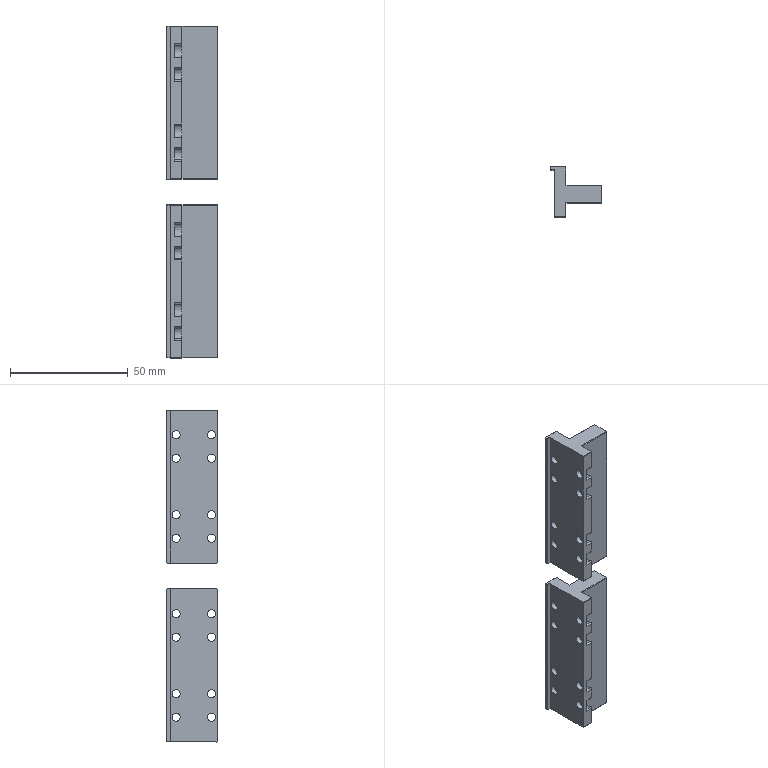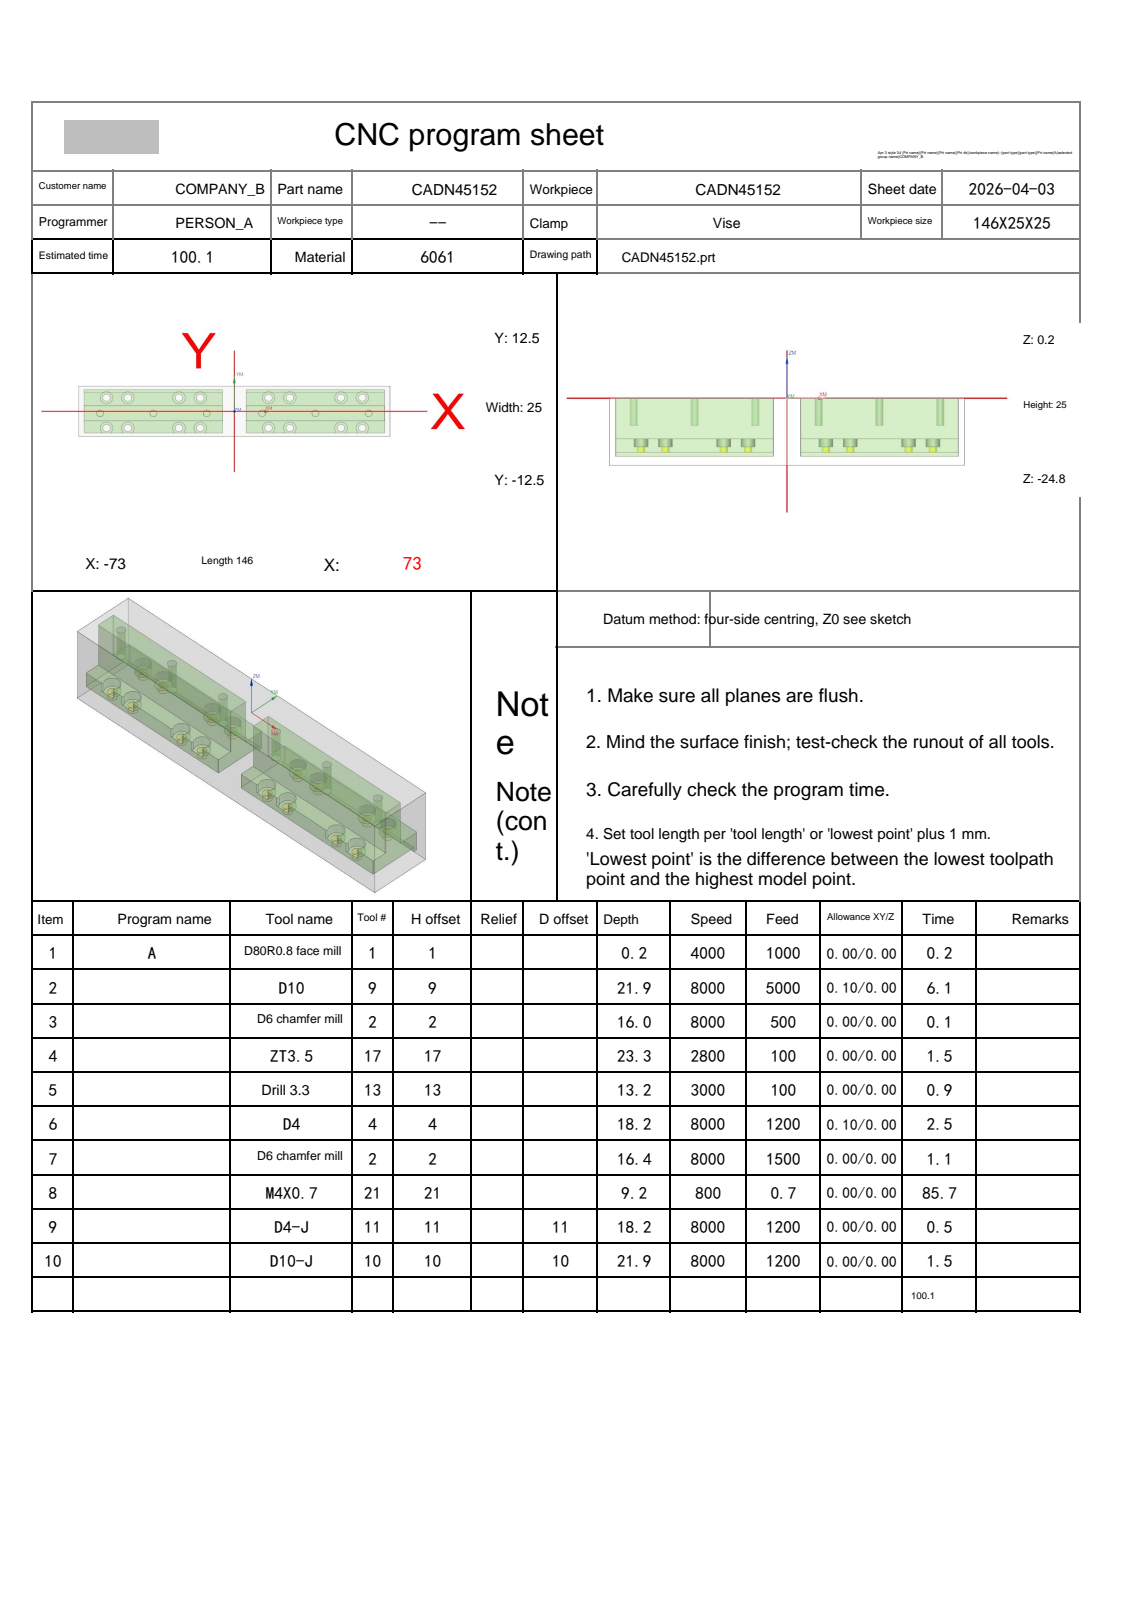NC program | NX | posted by the shop | part box 21.5 x 21.5 x 141 mm
Lines 36 to 798 of 7245:
N2 T09 M06
(D10  D=10. R=0. H=09 ce=0.10 di=0.00)
G00 G90 G54 X-38. Y-15.85 M03 S8000
G43 H09 Z20.
M08
Z.5
G01 X-70.3 Z.375 F5000.
G02 X-73.906 Y-14.356 Z.359 I0.0 J5.1
G01 X-74.106 Y-14.156 Z.358
G02 X-75.6 Y-10.55 Z.343 I3.606 J3.606
G01 Y10.55 Z.261
G02 X-74.106 Y14.156 Z.245 I5.1 J0.0
G01 X-73.906 Y14.356 Z.244
G02 X-70.3 Y15.85 Z.229 I3.606 J-3.606
G01 X-5.7 Z-.022
G02 X-2.094 Y14.356 Z-.037 I0.0 J-5.1
G01 X-1.894 Y14.156 Z-.038
G02 X-.4 Y10.55 Z-.054 I-3.606 J-3.606
G01 Y-10.55 Z-.136
G02 X-1.894 Y-14.156 Z-.151 I-5.1 J0.0
G01 X-2.094 Y-14.356 Z-.152
G02 X-5.7 Y-15.85 Z-.168 I-3.606 J3.606
G01 X-70.3 Z-.418
G02 X-73.906 Y-14.356 Z-.434 I0.0 J5.1
G01 X-74.106 Y-14.156 Z-.435
G02 X-75.6 Y-10.55 Z-.45 I3.606 J3.606
G01 Y10.55 Z-.532
G02 X-74.106 Y14.156 Z-.547 I5.1 J0.0
G01 X-73.906 Y14.356 Z-.549
G02 X-70.3 Y15.85 Z-.564 I3.606 J-3.606
G01 X-5.7 Z-.814
G02 X-2.094 Y14.356 Z-.83 I0.0 J-5.1
G01 X-1.894 Y14.156 Z-.831
G02 X-.4 Y10.55 Z-.847 I-3.606 J-3.606
G01 Y-10.55 Z-.928
G02 X-1.894 Y-14.156 Z-.944 I-5.1 J0.0
G01 X-2.094 Y-14.356 Z-.945
G02 X-5.7 Y-15.85 Z-.961 I-3.606 J3.606
G01 X-70.3 Z-1.211
G02 X-73.906 Y-14.356 Z-1.226 I0.0 J5.1
G01 X-74.106 Y-14.156 Z-1.228
G02 X-75.6 Y-10.55 Z-1.243 I3.606 J3.606
G01 Y10.55 Z-1.325
G02 X-74.106 Y14.156 Z-1.34 I5.1 J0.0
G01 X-73.906 Y14.356 Z-1.341
G02 X-70.3 Y15.85 Z-1.357 I3.606 J-3.606
G01 X-5.7 Z-1.607
G02 X-2.094 Y14.356 Z-1.623 I0.0 J-5.1
G01 X-1.894 Y14.156 Z-1.624
G02 X-.4 Y10.55 Z-1.639 I-3.606 J-3.606
G01 Y-10.55 Z-1.721
G02 X-1.894 Y-14.156 Z-1.737 I-5.1 J0.0
G01 X-2.094 Y-14.356 Z-1.738
G02 X-5.7 Y-15.85 Z-1.753 I-3.606 J3.606
G01 X-70.3 Z-2.004
G02 X-73.906 Y-14.356 Z-2.019 I0.0 J5.1
G01 X-74.106 Y-14.156 Z-2.02
G02 X-75.6 Y-10.55 Z-2.036 I3.606 J3.606
G01 Y10.55 Z-2.118
G02 X-74.106 Y14.156 Z-2.133 I5.1 J0.0
G01 X-73.906 Y14.356 Z-2.134
G02 X-70.3 Y15.85 Z-2.15 I3.606 J-3.606
G01 X-5.7 Z-2.4
G02 X-2.094 Y14.356 Z-2.416 I0.0 J-5.1
G01 X-1.894 Y14.156 Z-2.417
G02 X-.4 Y10.55 Z-2.432 I-3.606 J-3.606
G01 Y-10.55 Z-2.514
G02 X-1.894 Y-14.156 Z-2.53 I-5.1 J0.0
G01 X-2.094 Y-14.356 Z-2.531
G02 X-5.7 Y-15.85 Z-2.546 I-3.606 J3.606
G01 X-70.3 Z-2.797
G02 X-73.906 Y-14.356 Z-2.812 I0.0 J5.1
G01 X-74.106 Y-14.156 Z-2.813
G02 X-75.6 Y-10.55 Z-2.829 I3.606 J3.606
G01 Y10.55 Z-2.911
G02 X-74.106 Y14.156 Z-2.926 I5.1 J0.0
G01 X-73.906 Y14.356 Z-2.927
G02 X-70.3 Y15.85 Z-2.943 I3.606 J-3.606
G01 X-5.7 Z-3.193
G02 X-2.094 Y14.356 Z-3.209 I0.0 J-5.1
G01 X-1.894 Y14.156 Z-3.21
G02 X-.4 Y10.55 Z-3.225 I-3.606 J-3.606
G01 Y-10.55 Z-3.307
G02 X-1.894 Y-14.156 Z-3.322 I-5.1 J0.0
G01 X-2.094 Y-14.356 Z-3.324
G02 X-5.7 Y-15.85 Z-3.339 I-3.606 J3.606
G01 X-70.3 Z-3.589
G02 X-73.906 Y-14.356 Z-3.605 I0.0 J5.1
G01 X-74.106 Y-14.156 Z-3.606
G02 X-75.6 Y-10.55 Z-3.622 I3.606 J3.606
G01 Y10.55 Z-3.703
G02 X-74.106 Y14.156 Z-3.719 I5.1 J0.0
G01 X-73.906 Y14.356 Z-3.72
G02 X-70.3 Y15.85 Z-3.736 I3.606 J-3.606
G01 X-5.7 Z-3.986
G02 X-2.094 Y14.356 Z-4.001 I0.0 J-5.1
G01 X-1.894 Y14.156 Z-4.003
G02 X-.4 Y10.55 Z-4.018 I-3.606 J-3.606
G01 Y-10.55 Z-4.1
G02 X-1.894 Y-14.156 Z-4.115 I-5.1 J0.0
G01 X-2.094 Y-14.356 Z-4.116
G02 X-5.7 Y-15.85 Z-4.132 I-3.606 J3.606
G01 X-70.3 Z-4.382
G02 X-73.906 Y-14.356 Z-4.398 I0.0 J5.1
G01 X-74.106 Y-14.156 Z-4.399
G02 X-75.6 Y-10.55 Z-4.414 I3.606 J3.606
G01 Y10.55 Z-4.496
G02 X-74.106 Y14.156 Z-4.512 I5.1 J0.0
G01 X-73.906 Y14.356 Z-4.513
G02 X-70.3 Y15.85 Z-4.528 I3.606 J-3.606
G01 X-5.7 Z-4.779
G02 X-2.094 Y14.356 Z-4.794 I0.0 J-5.1
G01 X-1.894 Y14.156 Z-4.795
G02 X-.4 Y10.55 Z-4.811 I-3.606 J-3.606
G01 Y-10.55 Z-4.893
G02 X-1.894 Y-14.156 Z-4.908 I-5.1 J0.0
G01 X-2.094 Y-14.356 Z-4.909
G02 X-5.7 Y-15.85 Z-4.925 I-3.606 J3.606
G01 X-70.3 Z-5.175
G02 X-73.906 Y-14.356 Z-5.191 I0.0 J5.1
G01 X-74.106 Y-14.156 Z-5.192
G02 X-75.6 Y-10.55 Z-5.207 I3.606 J3.606
G01 Y10.55 Z-5.289
G02 X-74.106 Y14.156 Z-5.305 I5.1 J0.0
G01 X-73.906 Y14.356 Z-5.306
G02 X-70.3 Y15.85 Z-5.321 I3.606 J-3.606
G01 X-5.7 Z-5.572
G02 X-2.094 Y14.356 Z-5.587 I0.0 J-5.1
G01 X-1.894 Y14.156 Z-5.588
G02 X-.4 Y10.55 Z-5.604 I-3.606 J-3.606
G01 Y-10.55 Z-5.686
G02 X-1.894 Y-14.156 Z-5.701 I-5.1 J0.0
G01 X-2.094 Y-14.356 Z-5.702
G02 X-5.7 Y-15.85 Z-5.718 I-3.606 J3.606
G01 X-70.3 Z-5.968
G02 X-73.906 Y-14.356 Z-5.984 I0.0 J5.1
G01 X-74.106 Y-14.156 Z-5.985
G02 X-75.6 Y-10.55 Z-6. I3.606 J3.606
G01 Y10.55 Z-6.082
G02 X-74.106 Y14.156 Z-6.097 I5.1 J0.0
G01 X-73.906 Y14.356 Z-6.099
G02 X-70.3 Y15.85 Z-6.114 I3.606 J-3.606
G01 X-5.7 Z-6.364
G02 X-2.094 Y14.356 Z-6.38 I0.0 J-5.1
G01 X-1.894 Y14.156 Z-6.381
G02 X-.4 Y10.55 Z-6.397 I-3.606 J-3.606
G01 Y-10.55 Z-6.478
G02 X-1.894 Y-14.156 Z-6.494 I-5.1 J0.0
G01 X-2.094 Y-14.356 Z-6.495
G02 X-5.7 Y-15.85 Z-6.511 I-3.606 J3.606
G01 X-70.3 Z-6.761
G02 X-73.906 Y-14.356 Z-6.776 I0.0 J5.1
G01 X-74.106 Y-14.156 Z-6.778
G02 X-75.6 Y-10.55 Z-6.793 I3.606 J3.606
G01 Y10.55 Z-6.875
G02 X-74.106 Y14.156 Z-6.89 I5.1 J0.0
G01 X-73.906 Y14.356 Z-6.891
G02 X-70.3 Y15.85 Z-6.907 I3.606 J-3.606
G01 X-5.7 Z-7.157
G02 X-2.094 Y14.356 Z-7.173 I0.0 J-5.1
G01 X-1.894 Y14.156 Z-7.174
G02 X-.4 Y10.55 Z-7.189 I-3.606 J-3.606
G01 Y-10.55 Z-7.271
G02 X-1.894 Y-14.156 Z-7.287 I-5.1 J0.0
G01 X-2.094 Y-14.356 Z-7.288
G02 X-5.7 Y-15.85 Z-7.303 I-3.606 J3.606
G01 X-70.3 Z-7.554
G02 X-73.906 Y-14.356 Z-7.569 I0.0 J5.1
G01 X-74.106 Y-14.156 Z-7.57
G02 X-75.6 Y-10.55 Z-7.586 I3.606 J3.606
G01 Y10.55 Z-7.668
G02 X-74.106 Y14.156 Z-7.683 I5.1 J0.0
G01 X-73.906 Y14.356 Z-7.684
G02 X-70.3 Y15.85 Z-7.7 I3.606 J-3.606
G01 X-5.7 Z-7.95
G02 X-2.094 Y14.356 Z-7.966 I0.0 J-5.1
G01 X-1.894 Y14.156 Z-7.967
G02 X-.4 Y10.55 Z-7.982 I-3.606 J-3.606
G01 Y-10.55 Z-8.064
G02 X-1.894 Y-14.156 Z-8.08 I-5.1 J0.0
G01 X-2.094 Y-14.356 Z-8.081
G02 X-5.7 Y-15.85 Z-8.096 I-3.606 J3.606
G01 X-70.3 Z-8.347
G02 X-73.906 Y-14.356 Z-8.362 I0.0 J5.1
G01 X-74.106 Y-14.156 Z-8.363
G02 X-75.6 Y-10.55 Z-8.379 I3.606 J3.606
G01 Y10.55 Z-8.461
G02 X-74.106 Y14.156 Z-8.476 I5.1 J0.0
G01 X-73.906 Y14.356 Z-8.477
G02 X-70.3 Y15.85 Z-8.493 I3.606 J-3.606
G01 X-5.7 Z-8.743
G02 X-2.094 Y14.356 Z-8.759 I0.0 J-5.1
G01 X-1.894 Y14.156 Z-8.76
G02 X-.4 Y10.55 Z-8.775 I-3.606 J-3.606
G01 Y-10.55 Z-8.857
G02 X-1.894 Y-14.156 Z-8.872 I-5.1 J0.0
G01 X-2.094 Y-14.356 Z-8.874
G02 X-5.7 Y-15.85 Z-8.889 I-3.606 J3.606
G01 X-70.3 Z-9.139
G02 X-73.906 Y-14.356 Z-9.155 I0.0 J5.1
G01 X-74.106 Y-14.156 Z-9.156
G02 X-75.6 Y-10.55 Z-9.172 I3.606 J3.606
G01 Y10.55 Z-9.253
G02 X-74.106 Y14.156 Z-9.269 I5.1 J0.0
G01 X-73.906 Y14.356 Z-9.27
G02 X-70.3 Y15.85 Z-9.286 I3.606 J-3.606
G01 X-5.7 Z-9.536
G02 X-2.094 Y14.356 Z-9.551 I0.0 J-5.1
G01 X-1.894 Y14.156 Z-9.553
G02 X-.4 Y10.55 Z-9.568 I-3.606 J-3.606
G01 Y-10.55 Z-9.65
G02 X-1.894 Y-14.156 Z-9.665 I-5.1 J0.0
G01 X-2.094 Y-14.356 Z-9.666
G02 X-5.7 Y-15.85 Z-9.682 I-3.606 J3.606
G01 X-70.3 Z-9.932
G02 X-73.906 Y-14.356 Z-9.948 I0.0 J5.1
G01 X-74.106 Y-14.156 Z-9.949
G02 X-75.6 Y-10.55 Z-9.964 I3.606 J3.606
G01 Y10.55 Z-10.046
G02 X-74.106 Y14.156 Z-10.062 I5.1 J0.0
G01 X-73.906 Y14.356 Z-10.063
G02 X-70.3 Y15.85 Z-10.078 I3.606 J-3.606
G01 X-5.7 Z-10.329
G02 X-2.094 Y14.356 Z-10.344 I0.0 J-5.1
G01 X-1.894 Y14.156 Z-10.345
G02 X-.4 Y10.55 Z-10.361 I-3.606 J-3.606
G01 Y-10.55 Z-10.443
G02 X-1.894 Y-14.156 Z-10.458 I-5.1 J0.0
G01 X-2.094 Y-14.356 Z-10.459
G02 X-5.7 Y-15.85 Z-10.475 I-3.606 J3.606
G01 X-70.3 Z-10.725
G02 X-73.906 Y-14.356 Z-10.741 I0.0 J5.1
G01 X-74.106 Y-14.156 Z-10.742
G02 X-75.6 Y-10.55 Z-10.757 I3.606 J3.606
G01 Y10.55 Z-10.839
G02 X-74.106 Y14.156 Z-10.855 I5.1 J0.0
G01 X-73.906 Y14.356 Z-10.856
G02 X-70.3 Y15.85 Z-10.871 I3.606 J-3.606
G01 X-5.7 Z-11.122
G02 X-2.094 Y14.356 Z-11.137 I0.0 J-5.1
G01 X-1.894 Y14.156 Z-11.138
G02 X-.4 Y10.55 Z-11.154 I-3.606 J-3.606
G01 Y-10.55 Z-11.236
G02 X-1.894 Y-14.156 Z-11.251 I-5.1 J0.0
G01 X-2.094 Y-14.356 Z-11.252
G02 X-5.7 Y-15.85 Z-11.268 I-3.606 J3.606
G01 X-70.3 Z-11.518
G02 X-73.906 Y-14.356 Z-11.534 I0.0 J5.1
G01 X-74.106 Y-14.156 Z-11.535
G02 X-75.6 Y-10.55 Z-11.55 I3.606 J3.606
G01 Y10.55 Z-11.632
G02 X-74.106 Y14.156 Z-11.647 I5.1 J0.0
G01 X-73.906 Y14.356 Z-11.649
G02 X-70.3 Y15.85 Z-11.664 I3.606 J-3.606
G01 X-5.7 Z-11.914
G02 X-2.094 Y14.356 Z-11.93 I0.0 J-5.1
G01 X-1.894 Y14.156 Z-11.931
G02 X-.4 Y10.55 Z-11.947 I-3.606 J-3.606
G01 Y-10.55 Z-12.028
G02 X-1.894 Y-14.156 Z-12.044 I-5.1 J0.0
G01 X-2.094 Y-14.356 Z-12.045
G02 X-5.7 Y-15.85 Z-12.061 I-3.606 J3.606
G01 X-70.3 Z-12.311
G02 X-73.906 Y-14.356 Z-12.326 I0.0 J5.1
G01 X-74.106 Y-14.156 Z-12.328
G02 X-75.6 Y-10.55 Z-12.343 I3.606 J3.606
G01 Y10.55 Z-12.425
G02 X-74.106 Y14.156 Z-12.44 I5.1 J0.0
G01 X-73.906 Y14.356 Z-12.441
G02 X-70.3 Y15.85 Z-12.457 I3.606 J-3.606
G01 X-5.7 Z-12.707
G02 X-2.094 Y14.356 Z-12.723 I0.0 J-5.1
G01 X-1.894 Y14.156 Z-12.724
G02 X-.4 Y10.55 Z-12.739 I-3.606 J-3.606
G01 Y-10.55 Z-12.821
G02 X-1.894 Y-14.156 Z-12.837 I-5.1 J0.0
G01 X-2.094 Y-14.356 Z-12.838
G02 X-5.7 Y-15.85 Z-12.853 I-3.606 J3.606
G01 X-70.3 Z-13.104
G02 X-73.906 Y-14.356 Z-13.119 I0.0 J5.1
G01 X-74.106 Y-14.156 Z-13.12
G02 X-75.6 Y-10.55 Z-13.136 I3.606 J3.606
G01 Y10.55 Z-13.218
G02 X-74.106 Y14.156 Z-13.233 I5.1 J0.0
G01 X-73.906 Y14.356 Z-13.234
G02 X-70.3 Y15.85 Z-13.25 I3.606 J-3.606
G01 X-5.7 Z-13.5
G02 X-2.094 Y14.356 Z-13.516 I0.0 J-5.1
G01 X-1.894 Y14.156 Z-13.517
G02 X-.4 Y10.55 Z-13.532 I-3.606 J-3.606
G01 Y-10.55 Z-13.614
G02 X-1.894 Y-14.156 Z-13.63 I-5.1 J0.0
G01 X-2.094 Y-14.356 Z-13.631
G02 X-5.7 Y-15.85 Z-13.646 I-3.606 J3.606
G01 X-70.3 Z-13.897
G02 X-73.906 Y-14.356 Z-13.912 I0.0 J5.1
G01 X-74.106 Y-14.156 Z-13.913
G02 X-75.6 Y-10.55 Z-13.929 I3.606 J3.606
G01 Y10.55 Z-14.011
G02 X-74.106 Y14.156 Z-14.026 I5.1 J0.0
G01 X-73.906 Y14.356 Z-14.027
G02 X-70.3 Y15.85 Z-14.043 I3.606 J-3.606
G01 X-5.7 Z-14.293
G02 X-2.094 Y14.356 Z-14.309 I0.0 J-5.1
G01 X-1.894 Y14.156 Z-14.31
G02 X-.4 Y10.55 Z-14.325 I-3.606 J-3.606
G01 Y-10.55 Z-14.407
G02 X-1.894 Y-14.156 Z-14.422 I-5.1 J0.0
G01 X-2.094 Y-14.356 Z-14.424
G02 X-5.7 Y-15.85 Z-14.439 I-3.606 J3.606
G01 X-70.3 Z-14.689
G02 X-73.906 Y-14.356 Z-14.705 I0.0 J5.1
G01 X-74.106 Y-14.156 Z-14.706
G02 X-75.6 Y-10.55 Z-14.722 I3.606 J3.606
G01 Y10.55 Z-14.803
G02 X-74.106 Y14.156 Z-14.819 I5.1 J0.0
G01 X-73.906 Y14.356 Z-14.82
G02 X-70.3 Y15.85 Z-14.836 I3.606 J-3.606
G01 X-5.7 Z-15.086
G02 X-2.094 Y14.356 Z-15.101 I0.0 J-5.1
G01 X-1.894 Y14.156 Z-15.103
G02 X-.4 Y10.55 Z-15.118 I-3.606 J-3.606
G01 Y-10.55 Z-15.2
G02 X-1.894 Y-14.156 Z-15.215 I-5.1 J0.0
G01 X-2.094 Y-14.356 Z-15.216
G02 X-5.7 Y-15.85 Z-15.232 I-3.606 J3.606
G01 X-70.3 Z-15.482
G02 X-73.906 Y-14.356 Z-15.498 I0.0 J5.1
G01 X-74.106 Y-14.156 Z-15.499
G02 X-75.6 Y-10.55 Z-15.514 I3.606 J3.606
G01 Y10.55 Z-15.596
G02 X-74.106 Y14.156 Z-15.612 I5.1 J0.0
G01 X-73.906 Y14.356 Z-15.613
G02 X-70.3 Y15.85 Z-15.628 I3.606 J-3.606
G01 X-5.7 Z-15.879
G02 X-2.094 Y14.356 Z-15.894 I0.0 J-5.1
G01 X-1.894 Y14.156 Z-15.895
G02 X-.4 Y10.55 Z-15.911 I-3.606 J-3.606
G01 Y-10.55 Z-15.993
G02 X-1.894 Y-14.156 Z-16.008 I-5.1 J0.0
G01 X-2.094 Y-14.356 Z-16.009
G02 X-5.7 Y-15.85 Z-16.025 I-3.606 J3.606
G01 X-70.3 Z-16.275
G02 X-73.906 Y-14.356 Z-16.291 I0.0 J5.1
G01 X-74.106 Y-14.156 Z-16.292
G02 X-75.6 Y-10.55 Z-16.307 I3.606 J3.606
G01 Y10.55 Z-16.389
G02 X-74.106 Y14.156 Z-16.405 I5.1 J0.0
G01 X-73.906 Y14.356 Z-16.406
G02 X-70.3 Y15.85 Z-16.421 I3.606 J-3.606
G01 X-5.7 Z-16.672
G02 X-2.094 Y14.356 Z-16.687 I0.0 J-5.1
G01 X-1.894 Y14.156 Z-16.688
G02 X-.4 Y10.55 Z-16.704 I-3.606 J-3.606
G01 Y-10.55 Z-16.786
G02 X-1.894 Y-14.156 Z-16.801 I-5.1 J0.0
G01 X-2.094 Y-14.356 Z-16.802
G02 X-5.7 Y-15.85 Z-16.818 I-3.606 J3.606
G01 X-70.3 Z-17.068
G02 X-73.906 Y-14.356 Z-17.084 I0.0 J5.1
G01 X-74.106 Y-14.156 Z-17.085
G02 X-75.6 Y-10.55 Z-17.1 I3.606 J3.606
G01 Y10.55 Z-17.182
G02 X-74.106 Y14.156 Z-17.197 I5.1 J0.0
G01 X-73.906 Y14.356 Z-17.199
G02 X-70.3 Y15.85 Z-17.214 I3.606 J-3.606
G01 X-5.7 Z-17.464
G02 X-2.094 Y14.356 Z-17.48 I0.0 J-5.1
G01 X-1.894 Y14.156 Z-17.481
G02 X-.4 Y10.55 Z-17.497 I-3.606 J-3.606
G01 Y-10.55 Z-17.578
G02 X-1.894 Y-14.156 Z-17.594 I-5.1 J0.0
G01 X-2.094 Y-14.356 Z-17.595
G02 X-5.7 Y-15.85 Z-17.611 I-3.606 J3.606
G01 X-70.3 Z-17.861
G02 X-73.906 Y-14.356 Z-17.876 I0.0 J5.1
G01 X-74.106 Y-14.156 Z-17.878
G02 X-75.6 Y-10.55 Z-17.893 I3.606 J3.606
G01 Y10.55 Z-17.975
G02 X-74.106 Y14.156 Z-17.99 I5.1 J0.0
G01 X-73.906 Y14.356 Z-17.991
G02 X-70.3 Y15.85 Z-18.007 I3.606 J-3.606
G01 X-5.7 Z-18.257
G02 X-2.094 Y14.356 Z-18.273 I0.0 J-5.1
G01 X-1.894 Y14.156 Z-18.274
G02 X-.4 Y10.55 Z-18.289 I-3.606 J-3.606
G01 Y-10.55 Z-18.371
G02 X-1.894 Y-14.156 Z-18.387 I-5.1 J0.0
G01 X-2.094 Y-14.356 Z-18.388
G02 X-5.7 Y-15.85 Z-18.403 I-3.606 J3.606
G01 X-70.3 Z-18.654
G02 X-73.906 Y-14.356 Z-18.669 I0.0 J5.1
G01 X-74.106 Y-14.156 Z-18.67
G02 X-75.6 Y-10.55 Z-18.686 I3.606 J3.606
G01 Y10.55 Z-18.768
G02 X-74.106 Y14.156 Z-18.783 I5.1 J0.0
G01 X-73.906 Y14.356 Z-18.784
G02 X-70.3 Y15.85 Z-18.8 I3.606 J-3.606
G01 X-5.7 Z-19.05
G02 X-2.094 Y14.356 Z-19.066 I0.0 J-5.1
G01 X-1.894 Y14.156 Z-19.067
G02 X-.4 Y10.55 Z-19.082 I-3.606 J-3.606
G01 Y-10.55 Z-19.164
G02 X-1.894 Y-14.156 Z-19.18 I-5.1 J0.0
G01 X-2.094 Y-14.356 Z-19.181
G02 X-5.7 Y-15.85 Z-19.196 I-3.606 J3.606
G01 X-70.3 Z-19.447
G02 X-73.906 Y-14.356 Z-19.462 I0.0 J5.1
G01 X-74.106 Y-14.156 Z-19.463
G02 X-75.6 Y-10.55 Z-19.479 I3.606 J3.606
G01 Y10.55 Z-19.561
G02 X-74.106 Y14.156 Z-19.576 I5.1 J0.0
G01 X-73.906 Y14.356 Z-19.577
G02 X-70.3 Y15.85 Z-19.593 I3.606 J-3.606
G01 X-5.7 Z-19.843
G02 X-2.094 Y14.356 Z-19.859 I0.0 J-5.1
G01 X-1.894 Y14.156 Z-19.86
G02 X-.4 Y10.55 Z-19.875 I-3.606 J-3.606
G01 Y-10.55 Z-19.957
G02 X-1.894 Y-14.156 Z-19.972 I-5.1 J0.0
G01 X-2.094 Y-14.356 Z-19.974
G02 X-5.7 Y-15.85 Z-19.989 I-3.606 J3.606
G01 X-70.3 Z-20.239
G02 X-73.906 Y-14.356 Z-20.255 I0.0 J5.1
G01 X-74.106 Y-14.156 Z-20.256
G02 X-75.6 Y-10.55 Z-20.272 I3.606 J3.606
G01 Y10.55 Z-20.353
G02 X-74.106 Y14.156 Z-20.369 I5.1 J0.0
G01 X-73.906 Y14.356 Z-20.37
G02 X-70.3 Y15.85 Z-20.386 I3.606 J-3.606
G01 X-5.7 Z-20.636
G02 X-2.094 Y14.356 Z-20.651 I0.0 J-5.1
G01 X-1.894 Y14.156 Z-20.653
G02 X-.4 Y10.55 Z-20.668 I-3.606 J-3.606
G01 Y-10.55 Z-20.75
G02 X-1.894 Y-14.156 Z-20.765 I-5.1 J0.0
G01 X-2.094 Y-14.356 Z-20.766
G02 X-5.7 Y-15.85 Z-20.782 I-3.606 J3.606
G01 X-70.3 Z-21.032
G02 X-73.906 Y-14.356 Z-21.048 I0.0 J5.1
G01 X-74.106 Y-14.156 Z-21.049
G02 X-75.6 Y-10.55 Z-21.064 I3.606 J3.606
G01 Y10.55 Z-21.146
G02 X-74.106 Y14.156 Z-21.162 I5.1 J0.0
G01 X-73.906 Y14.356 Z-21.163
G02 X-70.3 Y15.85 Z-21.178 I3.606 J-3.606
G01 X-5.7 Z-21.429
G02 X-2.094 Y14.356 Z-21.444 I0.0 J-5.1
G01 X-1.894 Y14.156 Z-21.445
G02 X-.4 Y10.55 Z-21.461 I-3.606 J-3.606
G01 Y-10.55 Z-21.543
G02 X-1.894 Y-14.156 Z-21.558 I-5.1 J0.0
G01 X-2.094 Y-14.356 Z-21.559
G02 X-5.7 Y-15.85 Z-21.575 I-3.606 J3.606
G01 X-38. Z-21.7
X-70.3
G02 X-73.906 Y-14.356 I0.0 J5.1
G01 X-74.106 Y-14.156
G02 X-75.6 Y-10.55 I3.606 J3.606
G01 Y10.55
G02 X-74.106 Y14.156 I5.1 J0.0
G01 X-73.906 Y14.356
G02 X-70.3 Y15.85 I3.606 J-3.606
G01 X-5.7
G02 X-2.094 Y14.356 I0.0 J-5.1
G01 X-1.894 Y14.156
G02 X-.4 Y10.55 I-3.606 J-3.606
G01 Y-10.55
G02 X-1.894 Y-14.156 I-5.1 J0.0
G01 X-2.094 Y-14.356
G02 X-5.7 Y-15.85 I-3.606 J3.606
G01 X-38.
X-38.5
Z-20.7
G00 Z20.
X38.
Z.5
G01 X5.7 Z.375
G02 X2.094 Y-14.356 Z.359 I0.0 J5.1
G01 X1.894 Y-14.156 Z.358
G02 X.4 Y-10.55 Z.343 I3.606 J3.606
G01 Y10.55 Z.261
G02 X1.894 Y14.156 Z.245 I5.1 J0.0
G01 X2.094 Y14.356 Z.244
G02 X5.7 Y15.85 Z.229 I3.606 J-3.606
G01 X70.3 Z-.022
G02 X73.906 Y14.356 Z-.037 I0.0 J-5.1
G01 X74.106 Y14.156 Z-.038
G02 X75.6 Y10.55 Z-.054 I-3.606 J-3.606
G01 Y-10.55 Z-.136
G02 X74.106 Y-14.156 Z-.151 I-5.1 J0.0
G01 X73.906 Y-14.356 Z-.152
G02 X70.3 Y-15.85 Z-.168 I-3.606 J3.606
G01 X5.7 Z-.418
G02 X2.094 Y-14.356 Z-.434 I0.0 J5.1
G01 X1.894 Y-14.156 Z-.435
G02 X.4 Y-10.55 Z-.45 I3.606 J3.606
G01 Y10.55 Z-.532
G02 X1.894 Y14.156 Z-.547 I5.1 J0.0
G01 X2.094 Y14.356 Z-.549
G02 X5.7 Y15.85 Z-.564 I3.606 J-3.606
G01 X70.3 Z-.814
G02 X73.906 Y14.356 Z-.83 I0.0 J-5.1
G01 X74.106 Y14.156 Z-.831
G02 X75.6 Y10.55 Z-.847 I-3.606 J-3.606
G01 Y-10.55 Z-.928
G02 X74.106 Y-14.156 Z-.944 I-5.1 J0.0
G01 X73.906 Y-14.356 Z-.945
G02 X70.3 Y-15.85 Z-.961 I-3.606 J3.606
G01 X5.7 Z-1.211
G02 X2.094 Y-14.356 Z-1.226 I0.0 J5.1
G01 X1.894 Y-14.156 Z-1.228
G02 X.4 Y-10.55 Z-1.243 I3.606 J3.606
G01 Y10.55 Z-1.325
G02 X1.894 Y14.156 Z-1.34 I5.1 J0.0
G01 X2.094 Y14.356 Z-1.341
G02 X5.7 Y15.85 Z-1.357 I3.606 J-3.606
G01 X70.3 Z-1.607
G02 X73.906 Y14.356 Z-1.623 I0.0 J-5.1
G01 X74.106 Y14.156 Z-1.624
G02 X75.6 Y10.55 Z-1.639 I-3.606 J-3.606
G01 Y-10.55 Z-1.721
G02 X74.106 Y-14.156 Z-1.737 I-5.1 J0.0
G01 X73.906 Y-14.356 Z-1.738
G02 X70.3 Y-15.85 Z-1.753 I-3.606 J3.606
G01 X5.7 Z-2.004
G02 X2.094 Y-14.356 Z-2.019 I0.0 J5.1
G01 X1.894 Y-14.156 Z-2.02
G02 X.4 Y-10.55 Z-2.036 I3.606 J3.606
G01 Y10.55 Z-2.118
G02 X1.894 Y14.156 Z-2.133 I5.1 J0.0
G01 X2.094 Y14.356 Z-2.134
G02 X5.7 Y15.85 Z-2.15 I3.606 J-3.606
G01 X70.3 Z-2.4
G02 X73.906 Y14.356 Z-2.416 I0.0 J-5.1
G01 X74.106 Y14.156 Z-2.417
G02 X75.6 Y10.55 Z-2.432 I-3.606 J-3.606
G01 Y-10.55 Z-2.514
G02 X74.106 Y-14.156 Z-2.53 I-5.1 J0.0
G01 X73.906 Y-14.356 Z-2.531
G02 X70.3 Y-15.85 Z-2.546 I-3.606 J3.606
G01 X5.7 Z-2.797
G02 X2.094 Y-14.356 Z-2.812 I0.0 J5.1
G01 X1.894 Y-14.156 Z-2.813
G02 X.4 Y-10.55 Z-2.829 I3.606 J3.606
G01 Y10.55 Z-2.911
G02 X1.894 Y14.156 Z-2.926 I5.1 J0.0
G01 X2.094 Y14.356 Z-2.927
G02 X5.7 Y15.85 Z-2.943 I3.606 J-3.606
G01 X70.3 Z-3.193
G02 X73.906 Y14.356 Z-3.209 I0.0 J-5.1
G01 X74.106 Y14.156 Z-3.21
G02 X75.6 Y10.55 Z-3.225 I-3.606 J-3.606
G01 Y-10.55 Z-3.307
G02 X74.106 Y-14.156 Z-3.322 I-5.1 J0.0
G01 X73.906 Y-14.356 Z-3.324
G02 X70.3 Y-15.85 Z-3.339 I-3.606 J3.606
G01 X5.7 Z-3.589
G02 X2.094 Y-14.356 Z-3.605 I0.0 J5.1
G01 X1.894 Y-14.156 Z-3.606
G02 X.4 Y-10.55 Z-3.622 I3.606 J3.606
G01 Y10.55 Z-3.703
G02 X1.894 Y14.156 Z-3.719 I5.1 J0.0
G01 X2.094 Y14.356 Z-3.72
G02 X5.7 Y15.85 Z-3.736 I3.606 J-3.606
G01 X70.3 Z-3.986
G02 X73.906 Y14.356 Z-4.001 I0.0 J-5.1
G01 X74.106 Y14.156 Z-4.003
G02 X75.6 Y10.55 Z-4.018 I-3.606 J-3.606
G01 Y-10.55 Z-4.1
G02 X74.106 Y-14.156 Z-4.115 I-5.1 J0.0
G01 X73.906 Y-14.356 Z-4.116
G02 X70.3 Y-15.85 Z-4.132 I-3.606 J3.606
G01 X5.7 Z-4.382
G02 X2.094 Y-14.356 Z-4.398 I0.0 J5.1
G01 X1.894 Y-14.156 Z-4.399
G02 X.4 Y-10.55 Z-4.414 I3.606 J3.606
G01 Y10.55 Z-4.496
G02 X1.894 Y14.156 Z-4.512 I5.1 J0.0
G01 X2.094 Y14.356 Z-4.513
G02 X5.7 Y15.85 Z-4.528 I3.606 J-3.606
G01 X70.3 Z-4.779
G02 X73.906 Y14.356 Z-4.794 I0.0 J-5.1
G01 X74.106 Y14.156 Z-4.795
G02 X75.6 Y10.55 Z-4.811 I-3.606 J-3.606
G01 Y-10.55 Z-4.893
G02 X74.106 Y-14.156 Z-4.908 I-5.1 J0.0
G01 X73.906 Y-14.356 Z-4.909
G02 X70.3 Y-15.85 Z-4.925 I-3.606 J3.606
G01 X5.7 Z-5.175
G02 X2.094 Y-14.356 Z-5.191 I0.0 J5.1
G01 X1.894 Y-14.156 Z-5.192
G02 X.4 Y-10.55 Z-5.207 I3.606 J3.606
G01 Y10.55 Z-5.289
G02 X1.894 Y14.156 Z-5.305 I5.1 J0.0
G01 X2.094 Y14.356 Z-5.306
G02 X5.7 Y15.85 Z-5.321 I3.606 J-3.606
G01 X70.3 Z-5.572
G02 X73.906 Y14.356 Z-5.587 I0.0 J-5.1
G01 X74.106 Y14.156 Z-5.588
G02 X75.6 Y10.55 Z-5.604 I-3.606 J-3.606
G01 Y-10.55 Z-5.686
G02 X74.106 Y-14.156 Z-5.701 I-5.1 J0.0
G01 X73.906 Y-14.356 Z-5.702
G02 X70.3 Y-15.85 Z-5.718 I-3.606 J3.606
G01 X5.7 Z-5.968
G02 X2.094 Y-14.356 Z-5.984 I0.0 J5.1
G01 X1.894 Y-14.156 Z-5.985
G02 X.4 Y-10.55 Z-6. I3.606 J3.606
G01 Y10.55 Z-6.082
G02 X1.894 Y14.156 Z-6.097 I5.1 J0.0
G01 X2.094 Y14.356 Z-6.099
G02 X5.7 Y15.85 Z-6.114 I3.606 J-3.606
G01 X70.3 Z-6.364
G02 X73.906 Y14.356 Z-6.38 I0.0 J-5.1
G01 X74.106 Y14.156 Z-6.381
G02 X75.6 Y10.55 Z-6.397 I-3.606 J-3.606
G01 Y-10.55 Z-6.478
G02 X74.106 Y-14.156 Z-6.494 I-5.1 J0.0
G01 X73.906 Y-14.356 Z-6.495
G02 X70.3 Y-15.85 Z-6.511 I-3.606 J3.606
G01 X5.7 Z-6.761
G02 X2.094 Y-14.356 Z-6.776 I0.0 J5.1
G01 X1.894 Y-14.156 Z-6.778
G02 X.4 Y-10.55 Z-6.793 I3.606 J3.606
G01 Y10.55 Z-6.875
G02 X1.894 Y14.156 Z-6.89 I5.1 J0.0
G01 X2.094 Y14.356 Z-6.891
G02 X5.7 Y15.85 Z-6.907 I3.606 J-3.606
G01 X70.3 Z-7.157
G02 X73.906 Y14.356 Z-7.173 I0.0 J-5.1
G01 X74.106 Y14.156 Z-7.174
G02 X75.6 Y10.55 Z-7.189 I-3.606 J-3.606
G01 Y-10.55 Z-7.271
G02 X74.106 Y-14.156 Z-7.287 I-5.1 J0.0
G01 X73.906 Y-14.356 Z-7.288
G02 X70.3 Y-15.85 Z-7.303 I-3.606 J3.606
G01 X5.7 Z-7.554
G02 X2.094 Y-14.356 Z-7.569 I0.0 J5.1
G01 X1.894 Y-14.156 Z-7.57
G02 X.4 Y-10.55 Z-7.586 I3.606 J3.606
G01 Y10.55 Z-7.668
G02 X1.894 Y14.156 Z-7.683 I5.1 J0.0
G01 X2.094 Y14.356 Z-7.684
G02 X5.7 Y15.85 Z-7.7 I3.606 J-3.606
G01 X70.3 Z-7.95
G02 X73.906 Y14.356 Z-7.966 I0.0 J-5.1
G01 X74.106 Y14.156 Z-7.967
G02 X75.6 Y10.55 Z-7.982 I-3.606 J-3.606
G01 Y-10.55 Z-8.064
G02 X74.106 Y-14.156 Z-8.08 I-5.1 J0.0
G01 X73.906 Y-14.356 Z-8.081
G02 X70.3 Y-15.85 Z-8.096 I-3.606 J3.606
G01 X5.7 Z-8.347
G02 X2.094 Y-14.356 Z-8.362 I0.0 J5.1
G01 X1.894 Y-14.156 Z-8.363
G02 X.4 Y-10.55 Z-8.379 I3.606 J3.606
G01 Y10.55 Z-8.461
G02 X1.894 Y14.156 Z-8.476 I5.1 J0.0
G01 X2.094 Y14.356 Z-8.477
G02 X5.7 Y15.85 Z-8.493 I3.606 J-3.606
G01 X70.3 Z-8.743
G02 X73.906 Y14.356 Z-8.759 I0.0 J-5.1
G01 X74.106 Y14.156 Z-8.76
G02 X75.6 Y10.55 Z-8.775 I-3.606 J-3.606
G01 Y-10.55 Z-8.857
G02 X74.106 Y-14.156 Z-8.872 I-5.1 J0.0
G01 X73.906 Y-14.356 Z-8.874
G02 X70.3 Y-15.85 Z-8.889 I-3.606 J3.606
G01 X5.7 Z-9.139
G02 X2.094 Y-14.356 Z-9.155 I0.0 J5.1
G01 X1.894 Y-14.156 Z-9.156
G02 X.4 Y-10.55 Z-9.172 I3.606 J3.606
G01 Y10.55 Z-9.253
G02 X1.894 Y14.156 Z-9.269 I5.1 J0.0
G01 X2.094 Y14.356 Z-9.27
G02 X5.7 Y15.85 Z-9.286 I3.606 J-3.606
G01 X70.3 Z-9.536
G02 X73.906 Y14.356 Z-9.551 I0.0 J-5.1
G01 X74.106 Y14.156 Z-9.553
G02 X75.6 Y10.55 Z-9.568 I-3.606 J-3.606
G01 Y-10.55 Z-9.65
G02 X74.106 Y-14.156 Z-9.665 I-5.1 J0.0
G01 X73.906 Y-14.356 Z-9.666
G02 X70.3 Y-15.85 Z-9.682 I-3.606 J3.606
G01 X5.7 Z-9.932
G02 X2.094 Y-14.356 Z-9.948 I0.0 J5.1
G01 X1.894 Y-14.156 Z-9.949
G02 X.4 Y-10.55 Z-9.964 I3.606 J3.606
G01 Y10.55 Z-10.046
G02 X1.894 Y14.156 Z-10.062 I5.1 J0.0
G01 X2.094 Y14.356 Z-10.063
G02 X5.7 Y15.85 Z-10.078 I3.606 J-3.606
G01 X70.3 Z-10.329
G02 X73.906 Y14.356 Z-10.344 I0.0 J-5.1
G01 X74.106 Y14.156 Z-10.345
G02 X75.6 Y10.55 Z-10.361 I-3.606 J-3.606
G01 Y-10.55 Z-10.443
G02 X74.106 Y-14.156 Z-10.458 I-5.1 J0.0
G01 X73.906 Y-14.356 Z-10.459
G02 X70.3 Y-15.85 Z-10.475 I-3.606 J3.606
G01 X5.7 Z-10.725
G02 X2.094 Y-14.356 Z-10.741 I0.0 J5.1
G01 X1.894 Y-14.156 Z-10.742
G02 X.4 Y-10.55 Z-10.757 I3.606 J3.606
G01 Y10.55 Z-10.839
G02 X1.894 Y14.156 Z-10.855 I5.1 J0.0
G01 X2.094 Y14.356 Z-10.856
G02 X5.7 Y15.85 Z-10.871 I3.606 J-3.606
G01 X70.3 Z-11.122
G02 X73.906 Y14.356 Z-11.137 I0.0 J-5.1
G01 X74.106 Y14.156 Z-11.138
G02 X75.6 Y10.55 Z-11.154 I-3.606 J-3.606
G01 Y-10.55 Z-11.236
G02 X74.106 Y-14.156 Z-11.251 I-5.1 J0.0
G01 X73.906 Y-14.356 Z-11.252
G02 X70.3 Y-15.85 Z-11.268 I-3.606 J3.606
G01 X5.7 Z-11.518
G02 X2.094 Y-14.356 Z-11.534 I0.0 J5.1
G01 X1.894 Y-14.156 Z-11.535
G02 X.4 Y-10.55 Z-11.55 I3.606 J3.606
G01 Y10.55 Z-11.632
G02 X1.894 Y14.156 Z-11.647 I5.1 J0.0
G01 X2.094 Y14.356 Z-11.649
G02 X5.7 Y15.85 Z-11.664 I3.606 J-3.606
G01 X70.3 Z-11.914
G02 X73.906 Y14.356 Z-11.93 I0.0 J-5.1
G01 X74.106 Y14.156 Z-11.931
G02 X75.6 Y10.55 Z-11.947 I-3.606 J-3.606
G01 Y-10.55 Z-12.028
G02 X74.106 Y-14.156 Z-12.044 I-5.1 J0.0
G01 X73.906 Y-14.356 Z-12.045
G02 X70.3 Y-15.85 Z-12.061 I-3.606 J3.606
G01 X5.7 Z-12.311
G02 X2.094 Y-14.356 Z-12.326 I0.0 J5.1
G01 X1.894 Y-14.156 Z-12.328
G02 X.4 Y-10.55 Z-12.343 I3.606 J3.606
G01 Y10.55 Z-12.425
G02 X1.894 Y14.156 Z-12.44 I5.1 J0.0
G01 X2.094 Y14.356 Z-12.441
G02 X5.7 Y15.85 Z-12.457 I3.606 J-3.606
G01 X70.3 Z-12.707
G02 X73.906 Y14.356 Z-12.723 I0.0 J-5.1
G01 X74.106 Y14.156 Z-12.724
G02 X75.6 Y10.55 Z-12.739 I-3.606 J-3.606
G01 Y-10.55 Z-12.821
G02 X74.106 Y-14.156 Z-12.837 I-5.1 J0.0
G01 X73.906 Y-14.356 Z-12.838
G02 X70.3 Y-15.85 Z-12.853 I-3.606 J3.606
G01 X5.7 Z-13.104
G02 X2.094 Y-14.356 Z-13.119 I0.0 J5.1
G01 X1.894 Y-14.156 Z-13.12
G02 X.4 Y-10.55 Z-13.136 I3.606 J3.606
G01 Y10.55 Z-13.218
G02 X1.894 Y14.156 Z-13.233 I5.1 J0.0
G01 X2.094 Y14.356 Z-13.234
G02 X5.7 Y15.85 Z-13.25 I3.606 J-3.606
G01 X70.3 Z-13.5
G02 X73.906 Y14.356 Z-13.516 I0.0 J-5.1
G01 X74.106 Y14.156 Z-13.517
G02 X75.6 Y10.55 Z-13.532 I-3.606 J-3.606
G01 Y-10.55 Z-13.614
G02 X74.106 Y-14.156 Z-13.63 I-5.1 J0.0